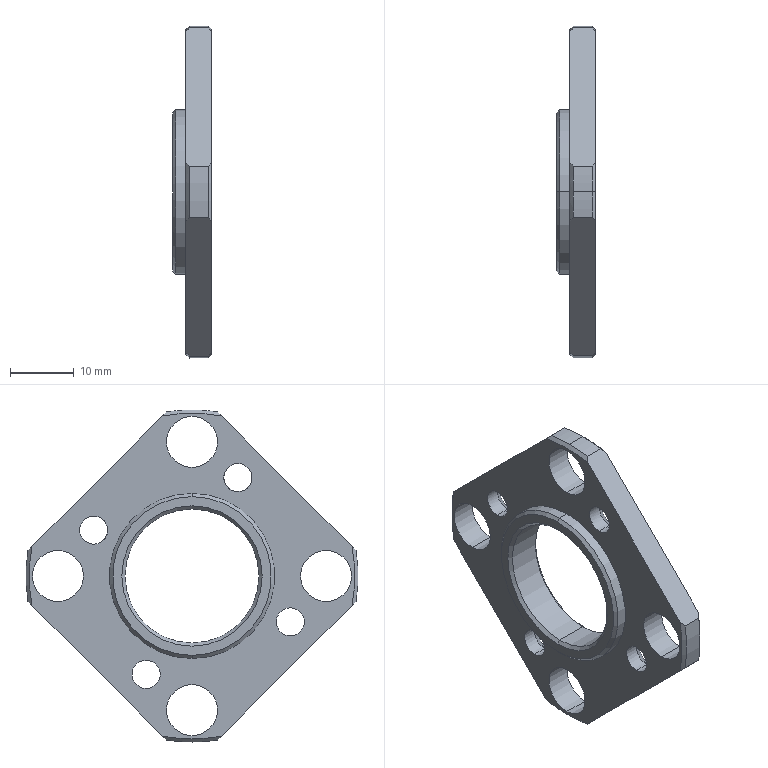Part | SolidWorks | features BaseBody 1 | 1 solid | 56 faces | box 6.1 x 52 x 52 mm | volume 4618 mm3 | cylinder 25 | cone 24 | plane 7 | commonest cylinder face diameters 4.4 x8 8 x8 52 x5 21 x2 25.85 x2